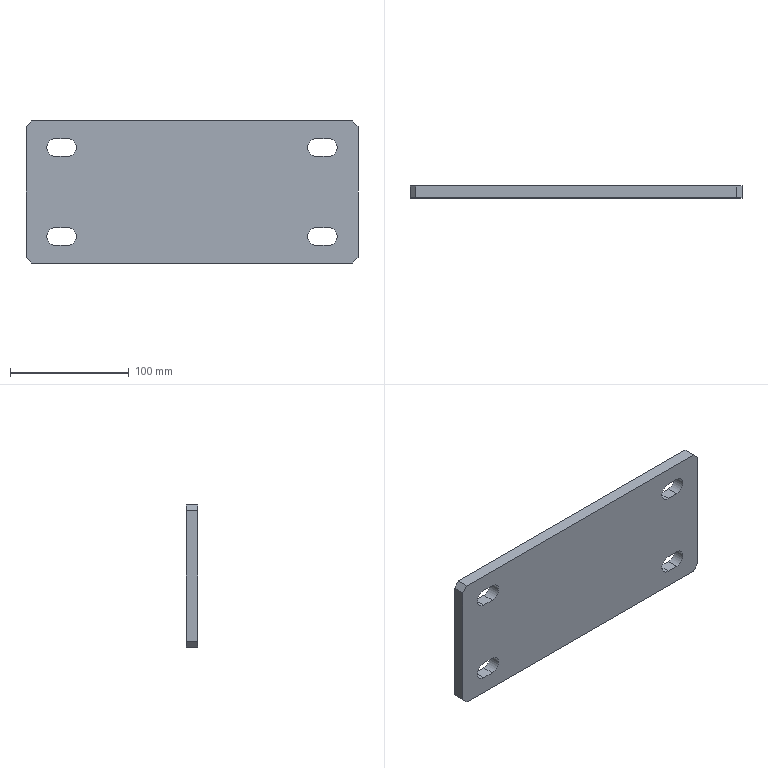Part | STEP file | Diagonal Brace连接Plate-45度 | 1 solid | 26 faces | box 280 x 10 x 120 mm | volume 322431 mm3 | plane 18 | cylinder 8 | commonest cylinder face diameters 15 x8